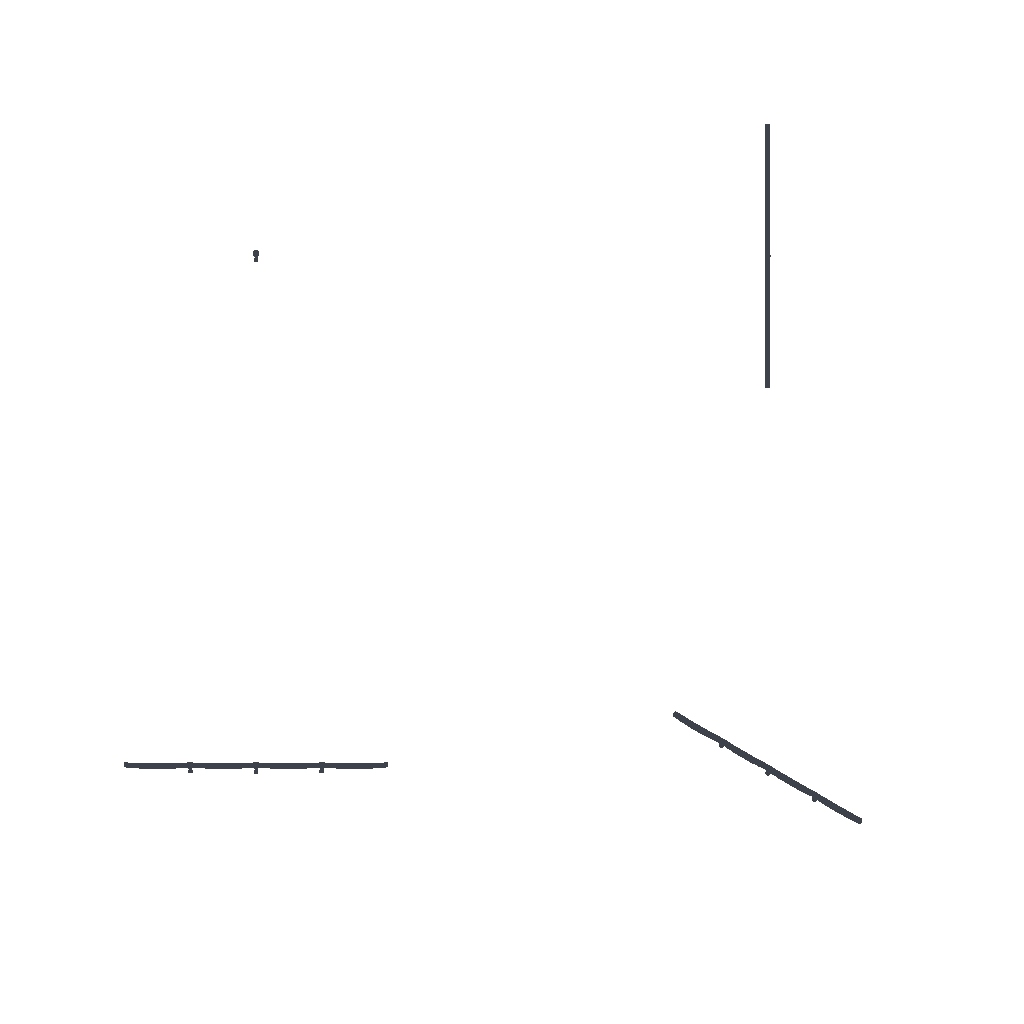Simulation study | abaqus
Set-up summary, first 274 of 540 lines:
category,name,step,type,value,unit,region
solver,abaqus,,Abaqus/CAE 2024
units,mm-N-s-tonne (MPa),,inferred,E=103600 density=6.967e-09
analysis,Step-G,,static,nlgeom=True; time_period=1
analysis,Step-F,,frequency (modal),n_modes=6
mesh,nodes,,,45210
mesh,elements,,,48438
element_type,B31,,,45138
element_type,T3D2,,,3300
material,conductor,,E,103600
material,conductor,,nu,0.3
material,conductor,,density,6.967e-09
material,ground,,E,103600
material,ground,,nu,0.3
material,ground,,density,6.967e-09
material,insulator,,E,206000
material,insulator,,nu,0.3
material,insulator,,density,1.9108e-09
material,insulator,,yield,2548
material,insulator,,cte,1.55e+07
material,insulator,,behaviors,plastic; expansion
material,steel-235,,E,206000
material,steel-235,,nu,0.3
material,steel-235,,density,7.85e-09
material,steel-235,,yield,235
material,steel-235,,behaviors,plastic
material,steel-355,,E,206000
material,steel-355,,nu,0.3
material,steel-355,,density,7.85e-09
material,steel-355,,yield,355
material,steel-355,,behaviors,plastic
material,steel-420,,E,206000
material,steel-420,,nu,0.3
material,steel-420,,density,7.85e-09
material,steel-420,,yield,420
material,steel-420,,behaviors,plastic
section,conductor,,solid section,,,_PickedSet2
section,conductor,,solid section,,,_PickedSet2
section,conductor,,solid section,,,_PickedSet2
section,ground,,solid section,,,_PickedSet2
section,steel-235,,beam section,,,_I1
section,steel-235,,beam section,,,_I2
section,steel-355,,beam section,,,_I3
section,steel-355,,beam section,,,_I4
section,steel-355,,beam section,,,_I5
section,steel-355,,beam section,,,_I6
section,steel-355,,beam section,,,_I7
section,steel-355,,beam section,,,_I8
section,steel-235,,beam section,,,_I9
section,steel-235,,beam section,,,_I10
section,steel-235,,beam section,,,_I11
section,steel-355,,beam section,,,_I12
section,steel-355,,beam section,,,_I13
section,steel-355,,beam section,,,_I14
section,steel-355,,beam section,,,_PickedSet581
section,steel-235,,beam section,,,_I16
section,steel-355,,beam section,,,_PickedSet580
section,steel-235,,beam section,,,_I18
section,steel-355,,beam section,,,_I19
section,steel-355,,beam section,,,_I20
section,steel-355,,beam section,,,_I21
section,steel-355,,beam section,,,_I22
section,steel-355,,beam section,,,_I23
section,steel-355,,beam section,,,_I24
section,steel-355,,beam section,,,_I25
section,steel-355,,beam section,,,_I26
section,steel-235,,beam section,,,_I27
section,steel-235,,beam section,,,_I28
section,steel-235,,beam section,,,_I29
section,steel-235,,beam section,,,_I30
section,steel-235,,beam section,,,_I31
section,steel-355,,beam section,,,_I32
section,steel-355,,beam section,,,_I33
section,steel-355,,beam section,,,_I34
section,steel-355,,beam section,,,_I35
section,steel-355,,beam section,,,_I36
section,steel-355,,beam section,,,_I37
section,steel-355,,beam section,,,_I38
section,steel-355,,beam section,,,_I39
section,steel-355,,beam section,,,_I40
section,steel-355,,beam section,,,_I41
section,steel-235,,beam section,,,_I42
section,steel-235,,beam section,,,_PickedSet576
section,steel-235,,beam section,,,_PickedSet577
section,steel-355,,beam section,,,_I45
section,steel-355,,beam section,,,_I46
section,steel-235,,beam section,,,_I47
section,steel-235,,beam section,,,_PickedSet579
section,steel-355,,beam section,,,_I49
section,steel-355,,beam section,,,_I50
section,steel-235,,beam section,,,_PickedSet603
section,steel-235,,beam section,,,_PickedSet604
section,steel-235,,beam section,,,_I53
section,steel-235,,beam section,,,_I54
section,steel-355,,beam section,,,_I55
section,steel-235,,beam section,,,_I56
section,steel-235,,beam section,,,_I57
section,steel-355,,beam section,,,_I58
section,steel-355,,beam section,,,_I59
section,steel-235,,beam section,,,_I60
section,steel-235,,beam section,,,_I61
section,steel-355,,beam section,,,_I62
section,steel-355,,beam section,,,_I63
section,steel-235,,beam section,,,_I64
section,steel-355,,beam section,,,_I65
section,steel-355,,beam section,,,_I66
section,steel-355,,beam section,,,_I67
section,steel-235,,beam section,,,_I68
section,steel-355,,beam section,,,_I69
section,steel-235,,beam section,,,_I70
section,steel-235,,beam section,,,_I71
section,steel-355,,beam section,,,_I72
section,steel-235,,beam section,,,_PickedSet563
section,steel-355,,beam section,,,_I74
section,steel-235,,beam section,,,_I75
section,steel-235,,beam section,,,_I76
section,steel-235,,beam section,,,_I77
section,steel-355,,beam section,,,_I78
section,steel-355,,beam section,,,_PickedSet557
section,steel-355,,beam section,,,_PickedSet558
section,steel-235,,beam section,,,_I81
section,steel-355,,beam section,,,_I82
section,steel-355,,beam section,,,_I83
section,steel-235,,beam section,,,_I84
section,steel-355,,beam section,,,_I85
section,steel-355,,beam section,,,_I86
section,steel-355,,beam section,,,_I87
section,steel-235,,beam section,,,_I88
section,steel-235,,beam section,,,_I89
section,steel-235,,beam section,,,_I90
section,steel-355,,beam section,,,_I91
section,steel-235,,beam section,,,_I92
section,steel-235,,beam section,,,_I93
section,steel-235,,beam section,,,_I94
section,steel-235,,beam section,,,_I95
section,steel-235,,beam section,,,_I96
section,steel-235,,beam section,,,_I97
section,steel-355,,beam section,,,_I98
section,steel-355,,beam section,,,_I99
section,steel-355,,beam section,,,_I100
section,steel-355,,beam section,,,_I101
section,steel-355,,beam section,,,_I102
section,steel-355,,beam section,,,_I103
section,steel-235,,beam section,,,_I104
section,steel-235,,beam section,,,_I105
section,steel-355,,beam section,,,_I106
section,steel-235,,beam section,,,_I107
section,steel-355,,beam section,,,_I108
section,steel-235,,beam section,,,_I109
section,steel-235,,beam section,,,_I110
section,steel-355,,beam section,,,_I111
section,steel-235,,beam section,,,_I112
section,steel-235,,beam section,,,_I113
section,steel-355,,beam section,,,_I114
section,steel-355,,beam section,,,_I115
section,steel-235,,beam section,,,_I116
section,steel-235,,beam section,,,_I117
section,steel-235,,beam section,,,_I118
section,steel-235,,beam section,,,_I119
section,steel-235,,beam section,,,_I120
section,steel-235,,beam section,,,_I121
section,steel-235,,beam section,,,_I122
section,steel-235,,beam section,,,_I123
section,steel-355,,beam section,,,_I124
section,steel-420,,beam section,,,_I125
section,steel-355,,beam section,,,_I126
section,steel-355,,beam section,,,_I127
section,steel-355,,beam section,,,_I128
section,steel-420,,beam section,,,_I129
section,steel-355,,beam section,,,_I130
section,steel-235,,beam section,,,_I131
section,steel-235,,beam section,,,_I132
section,steel-355,,beam section,,,_I133
section,steel-355,,beam section,,,_I134
section,steel-235,,beam section,,,_I135
section,steel-235,,beam section,,,_I136
section,steel-235,,beam section,,,_I137
section,steel-235,,beam section,,,_I138
section,steel-235,,beam section,,,_I139
section,steel-235,,beam section,,,_I140
section,steel-235,,beam section,,,_I141
section,steel-355,,beam section,,,_I142
section,steel-235,,beam section,,,_I143
section,steel-235,,beam section,,,_I144
section,steel-235,,beam section,,,_I145
section,steel-235,,beam section,,,_I146
section,steel-235,,beam section,,,_I147
section,steel-235,,beam section,,,_I148
section,steel-355,,beam section,,,_I149
section,steel-235,,beam section,,,_I150
section,steel-235,,beam section,,,_I151
section,steel-235,,beam section,,,_I152
section,steel-235,,beam section,,,_I153
section,steel-235,,beam section,,,_I154
section,steel-235,,beam section,,,_I155
section,steel-235,,beam section,,,_I156
section,steel-235,,beam section,,,_I157
section,steel-355,,beam section,,,_I158
section,steel-235,,beam section,,,_I159
section,steel-235,,beam section,,,_I160
section,steel-235,,beam section,,,_I161
section,steel-355,,beam section,,,_I162
section,steel-235,,beam section,,,_I163
section,steel-235,,beam section,,,_I164
section,steel-355,,beam section,,,_I165
section,steel-235,,beam section,,,_I166
section,steel-355,,beam section,,,_I167
section,steel-355,,beam section,,,_I168
section,steel-355,,beam section,,,_I169
section,steel-235,,beam section,,,_I170
section,steel-235,,beam section,,,_I171
section,steel-355,,beam section,,,_I172
section,steel-355,,beam section,,,_I173
section,steel-235,,beam section,,,_I174
section,steel-355,,beam section,,,_I175
section,steel-235,,beam section,,,_I176
section,steel-235,,beam section,,,_I177
section,steel-235,,beam section,,,_I178
section,steel-235,,beam section,,,_I179
section,steel-235,,beam section,,,_I180
section,steel-355,,beam section,,,_I181
section,steel-355,,beam section,,,_I182
section,steel-235,,beam section,,,_I183
section,steel-235,,beam section,,,_I184
section,steel-235,,beam section,,,_I185
section,steel-355,,beam section,,,_I186
section,steel-235,,beam section,,,_I187
section,steel-235,,beam section,,,_I188
section,steel-235,,beam section,,,_I189
section,steel-235,,beam section,,,_I190
section,steel-235,,beam section,,,_I191
section,steel-355,,beam section,,,_I192
section,steel-235,,beam section,,,_I193
section,steel-235,,beam section,,,_I194
section,steel-355,,beam section,,,_I195
section,steel-355,,beam section,,,_I196
section,steel-235,,beam section,,,_PickedSet553
section,steel-235,,beam section,,,_I198
section,steel-355,,beam section,,,_I199
section,steel-235,,beam section,,,_I200
section,steel-355,,beam section,,,_I201
section,steel-235,,beam section,,,_I202
section,steel-235,,beam section,,,_I203
section,steel-355,,beam section,,,_I204
section,steel-420,,beam section,,,_I205
section,steel-355,,beam section,,,_PickedSet542
section,steel-355,,beam section,,,_I207
section,steel-235,,beam section,,,_PickedSet535
section,steel-235,,beam section,,,_PickedSet534
section,steel-355,,beam section,,,_I210
section,steel-420,,beam section,,,_I211
section,steel-355,,beam section,,,_I212
section,steel-235,,beam section,,,_PickedSet536
section,steel-420,,beam section,,,_I214
section,steel-355,,beam section,,,_I215
section,steel-420,,beam section,,,_I216
section,steel-235,,beam section,,,_I217
section,steel-235,,beam section,,,_PickedSet514
section,steel-235,,beam section,,,_I219
section,steel-235,,beam section,,,_I220
section,steel-235,,beam section,,,_I221
section,steel-235,,beam section,,,_I222
section,steel-235,,beam section,,,_I223
section,steel-235,,beam section,,,_I224
section,steel-355,,beam section,,,_I225
section,steel-420,,beam section,,,_I226
section,steel-235,,beam section,,,_I227
section,steel-235,,beam section,,,_I228
section,steel-355,,beam section,,,_I229
section,steel-235,,beam section,,,_I230
section,steel-235,,beam section,,,_I231
section,steel-235,,beam section,,,_I232
section,steel-235,,beam section,,,_I233
section,steel-235,,beam section,,,_I234
Abaqus input file, long lists of numbers shortened, first 686 of 3467 lines:
*Heading
** Job name: deck Model name: Model-1
** Generated by: Abaqus/CAE 2024
*Preprint, echo=NO, model=NO, history=NO, contact=NO
**
** PARTS
**
*Part, name=conductor-1
*Node
      1,    -199300.5,   5545.472,           0.
      2,  -195326.375,   5107.127,           0.
** (99 more lines like these left out)
*Element, type=T3D2
  1,   1,   2
  2,   2,   3
** (98 more lines like these left out)
*Nset, nset=_PickedSet2, internal, generate
   1,  101,    1
*Elset, elset=_PickedSet2, internal, generate
   1,  100,    1
** Section: conductor
*Solid Section, elset=_PickedSet2, material=conductor
425.24,
*End Part
**
*Part, name=conductor-2
*Node
      1,    -199305.5,   5545.75,           0.
      2,  -195331.281,   5107.384,           0.
** (99 more lines like these left out)
*Element, type=T3D2
  1,   1,   2
  2,   2,   3
** (98 more lines like these left out)
*Nset, nset=_PickedSet2, internal, generate
   1,  101,    1
*Elset, elset=_PickedSet2, internal, generate
   1,  100,    1
** Section: conductor
*Solid Section, elset=_PickedSet2, material=conductor
425.24,
*End Part
**
*Part, name=conductor-3
*Node
      1,  -199120.688,   5535.459,           0.
      2,  -195150.125,   5097.904,           0.
** (99 more lines like these left out)
*Element, type=T3D2
  1,   1,   2
  2,   2,   3
** (98 more lines like these left out)
*Nset, nset=_PickedSet2, internal, generate
   1,  101,    1
*Elset, elset=_PickedSet2, internal, generate
   1,  100,    1
** Section: conductor
*Solid Section, elset=_PickedSet2, material=conductor
425.24,
*End Part
**
*Part, name=ground
*Node
      1,  -199400.406,    2214.142,           0.
      2,  -195410.953,   2038.688,           0.
** (99 more lines like these left out)
*Element, type=T3D2
  1,   1,   2
  2,   2,   3
** (98 more lines like these left out)
*Nset, nset=_PickedSet2, internal, generate
   1,  101,    1
*Elset, elset=_PickedSet2, internal, generate
   1,  100,    1
** Section: ground
*Solid Section, elset=_PickedSet2, material=ground
148.07,
*End Part
**
*Part, name=shudianta
*Node
      1,  -2504.131,   915.163,       45600.
      2,       -3822.,   683.185,   46098.164
** (13957 more lines like these left out)
*Element, type=B31
1,   1, 715
2, 715, 716
** (15044 more lines like these left out)
*Nset, nset=Wire-2-Set-1
   506,   511,   515,   517,   550,   552,   556,   557,   570,   573,   575,   576,   584,   586,   587,   589
   593,   594,   596,   600,   607,   619,   620,   622,   627,   628,   641,   644,   646,   648,   653,   655
** (33 more lines like these left out)
*Elset, elset=Wire-2-Set-1
  8915,  8916,  8917,  8918,  8919,  8920,  8921,  8922,  8923,  8924, 10205, 10206, 10207, 10208, 10209, 10210
 10211, 10212, 10213, 10214, 10215, 10216, 10217, 10218, 10219, 10220, 10221, 10222, 10223, 10224, 10478, 10479
** (33 more lines like these left out)
*Nset, nset=Wire-3-Set-1
   503,   516,   517,   558,   559,   560,   561,   563,   570,   571,   573,   575,   580,   581,   582,   583
   584,   586,   587,   589,   590,   591,   593,   594,   596,   600,   601,   619,   620,   622,   623,   624
** (37 more lines like these left out)
*Elset, elset=Wire-3-Set-1
  8939,  8940,  8941,  8942,  8943,  8944,  8945,  8946,  8947,  8948,  8949,  8950, 10239, 10240, 10241, 10242
 10243, 10244, 10245, 10246, 10247, 10248, 10249, 10250, 10251, 10252, 10253, 10254, 10255, 10256, 10257, 10258
** (35 more lines like these left out)
*Nset, nset=Wire-4-Set-1
   516,   558,   559,   560,   561,   562,   563,   571,   581,   582,   583,   591,   592,   601,   602,   623
   624,   626,   638,   643,   649,   650,   651,   652,   668,   669,   670,   683,   684,   690,   698,   705
** (13 more lines like these left out)
*Elset, elset=Wire-4-Set-1
 10263, 10264, 10265, 10266, 10267, 10268, 10269, 10270, 10271, 10272, 10273, 10274, 10275, 10276, 10285, 10286
 10287, 10288, 10297, 10298, 10299, 10300, 10301, 10302, 10303, 10304, 10305, 10306, 10698, 10699, 10700, 10701
** (12 more lines like these left out)
*Nset, nset=Wire-5-Set-1
   506,   507,   508,   509,   510,   511,   573,   574,   575,   641,   642,   644,   646,   688,   689,   691
   692,   693,   694,   697,   707,  8321,  8322,  8323,  8324,  8325,  8326,  8327,  8328,  8329,  8330,  8340
** (13 more lines like these left out)
*Elset, elset=Wire-5-Set-1
  8826,  8827,  8828,  8829,  8830,  8831,  8832,  8833,  8834,  8835,  8836,  8847,  8848,  8849,  8850,  8851
  8852,  8853,  8854,  8855,  8856,  8857,  8858,  8859,  8860,  8861,  8862,  8863,  8864,  8865,  8866,  8867
** (13 more lines like these left out)
*Nset, nset=Wire-6-Set-1
   507,   508,   510,   557,   574,   576,  8331,  8332,  8333,  8334,  8335,  8336,  8337,  8338,  8339,  9960
  9961,  9962,  9963,  9964,  9965,  9966, 11238, 11239, 11240, 11241, 11242, 11243, 11244, 11245, 11246, 11247
** (2 more lines like these left out)
*Elset, elset=Wire-6-Set-1
  8837,  8838,  8839,  8840,  8841,  8842,  8843,  8844,  8845,  8846, 10620, 10621, 10622, 10623, 10624, 10625
 10626, 10627, 12024, 12025, 12026, 12027, 12028, 12029, 12030, 12031, 12032, 12033, 12034, 12168, 12169, 12170
** (2 more lines like these left out)
*Nset, nset=Wire-7-Set-1
   511,   517,   518,   577,   584,   585,   586,   587,   588,   589,   593,   594,   595,   596,   597,   600
   607,   659,   661,   702,   703,  8434,  8435,  8436,  8437,  8438,  8439,  8440,  9976,  9977,  9978,  9979
** (13 more lines like these left out)
*Elset, elset=Wire-7-Set-1
  8951,  8952,  8953,  8954,  8955,  8956,  8957,  8958, 10638, 10639, 10640, 10641, 10642, 10643, 10644, 10645
 10646, 10647, 10648, 10735, 10736, 10737, 10738, 10739, 10740, 10741, 10742, 10743, 10744, 10745, 10746, 10747
** (13 more lines like these left out)
*Nset, nset=Wire-8-Set-1
   515,   518,   577,   660,   702,   703,  8441,  8442,  8443,  8444,  8445,  8446,  8447,  8448,  8449,  8450
  9986,  9987,  9988,  9989,  9990,  9991,  9992, 10330, 10331, 10332, 10333, 10334, 10335, 10336, 10337, 10338
** (2 more lines like these left out)
*Elset, elset=Wire-8-Set-1
  8959,  8960,  8961,  8962,  8963,  8964,  8965,  8966,  8967,  8968,  8969, 10649, 10650, 10651, 10652, 10653
 10654, 10655, 10656, 11031, 11032, 11033, 11034, 11035, 11036, 11037, 11038, 11039, 11040, 14288, 14289, 14290
** (2 more lines like these left out)
*Nset, nset=Wire-9-Set-1
   550,   607,   615,   616,   617,   618,   619,   620,   621,   622,   627,   666,   671,   672,   677,   678
   679,   680,   681,   682,   706, 10610, 10611, 10612, 10613, 10614, 10615, 10616, 10617, 10618, 10619, 10629
** (13 more lines like these left out)
*Elset, elset=Wire-9-Set-1
 11338, 11339, 11340, 11341, 11342, 11343, 11344, 11345, 11346, 11347, 11348, 11359, 11360, 11361, 11362, 11363
 11364, 11365, 11366, 11367, 11368, 11369, 11370, 11371, 11372, 11373, 11374, 11375, 11376, 11377, 11378, 11379
** (13 more lines like these left out)
*Nset, nset=Wire-10-Set-1
   615,   616,   618,   628,   665,   666, 10620, 10621, 10622, 10623, 10624, 10625, 10626, 10627, 10628, 10768
 10769, 10770, 10771, 10772, 10773, 10774, 12204, 12205, 12206, 12207, 12208, 12209, 12210, 12287, 12288, 12289
** (2 more lines like these left out)
*Elset, elset=Wire-10-Set-1
 11349, 11350, 11351, 11352, 11353, 11354, 11355, 11356, 11357, 11358, 11512, 11513, 11514, 11515, 11516, 11517
 11518, 11519, 13088, 13089, 13090, 13091, 13092, 13093, 13094, 13095, 13179, 13180, 13181, 13182, 13183, 13184
** (2 more lines like these left out)
*Nset, nset=Wire-11-Set-1
   506,   550,   551,   553,   554,   555,   569,   570,   648,   653,   655,   656,   685,   686,   687,   699
   700,   701,   709,   711,   713,  9531,  9532,  9533,  9534,  9535,  9536,  9537,  9538,  9539,  9540,  9558
** (13 more lines like these left out)
*Elset, elset=Wire-11-Set-1
 10148, 10149, 10150, 10151, 10152, 10153, 10154, 10155, 10156, 10157, 10158, 10178, 10179, 10180, 10181, 10182
 10183, 10184, 10185, 10186, 10187, 10188, 10189, 10190, 10191, 10192, 10193, 10459, 10460, 10461, 10462, 10463
** (13 more lines like these left out)
*Nset, nset=Wire-12-Set-1
   551,   552,   553,   555,   556,   569,  9541,  9542,  9543,  9544,  9545,  9546,  9547,  9548,  9549,  9550
  9551,  9552,  9553,  9554,  9555,  9556,  9557,  9572,  9573,  9574,  9575,  9576,  9577,  9578,  9579,  9580
** (2 more lines like these left out)
*Elset, elset=Wire-12-Set-1
 10159, 10160, 10161, 10162, 10163, 10164, 10165, 10166, 10167, 10168, 10169, 10170, 10171, 10172, 10173, 10174
 10175, 10176, 10177, 10194, 10195, 10196, 10197, 10198, 10199, 10200, 10201, 10202, 10203, 10204, 10470, 10471
** (2 more lines like these left out)
*Nset, nset=Wire-13-Set-1
   504,   505,   506,   511,   512,   514,   550,   566,   568,   578,   579,   598,   607,   608,   609,   611
   612,   613,   614,   634,   635,   636,   639,   647,  8312,  8313,  8314,  8315,  8316,  8317,  8318,  8319
** (13 more lines like these left out)
*Elset, elset=Wire-13-Set-1
  8816,  8817,  8818,  8819,  8820,  8821,  8822,  8823,  8824,  8825,  8877,  8878,  8879,  8880,  8881,  8882
  8883,  8884,  8885,  8886,  8905,  8906,  8907,  8908,  8909,  8910,  8911,  8912,  8913,  8914, 10449, 10450
** (13 more lines like these left out)
*Nset, nset=Wire-14-Set-1
   503,   504,   505,   512,   513,   514,   566,   567,   568,   578,   579,   580,   598,   608,   609,   610
   611,   612,   613,   614,   630,   632,   634,   635,   636,   637,   639,   647,  8307,  8308,  8309,  8310
** (10 more lines like these left out)
*Elset, elset=Wire-14-Set-1
  8810,  8811,  8812,  8813,  8814,  8815,  8887,  8888,  8889,  8890,  8891,  8892,  8893,  8894,  8895,  8896
  8897,  8898,  8899,  8900,  8901,  8902,  8903,  8904, 10415, 10416, 10417, 10418, 10419, 10420, 10440, 10441
** (9 more lines like these left out)
*Nset, nset=Wire-15-Set-1
   506,   511,   513,   550,   567,   607,   610,   637,  9792,  9793,  9794,  9795, 10207, 10208, 10209, 10210
 12249, 12250, 12251, 12252, 12735, 12736, 12737, 12738
*Elset, elset=Wire-15-Set-1
 10435, 10436, 10437, 10438, 10439, 10895, 10896, 10897, 10898, 10899, 13137, 13138, 13139, 13140, 13141, 13675
 13676, 13677, 13678, 13679
*Nset, nset=Wire-18-Set-1
   436,   451,   452,   469,   470,   471,   473,   477,   483,   484,   487,   488,   489,   490,   492,   494
   495,   496,   498,   499,   524,   525,   529,   535,  7425,  7426,  7427,  7428,  7429,  7430,  7431,  7432
** (8 more lines like these left out)
*Elset, elset=Wire-18-Set-1
  7823,  7824,  7825,  7826,  7827,  7828,  7829,  7830,  7831,  8365,  8366,  8367,  8368,  8369,  8370,  8371
  8372,  8373,  8374,  8375,  8376,  8377,  8378,  8379,  8380,  8381,  8382,  8383,  8384,  8587,  8588,  8589
** (8 more lines like these left out)
*Nset, nset=Wire-19-Set-1
   456,   502,   506,   511,   538,   548,   549,   550,   565,   572,   605,   606,   607,   629,   631,   667
  8264,  8265,  8266,  8267,  8268,  8269,  8270,  8271,  8272,  8273,  8274,  8275,  8276,  8277,  9503,  9504
** (13 more lines like these left out)
*Elset, elset=Wire-19-Set-1
  8764,  8765,  8766,  8767,  8768,  8769,  8770,  8771,  8772,  8773,  8774,  8775,  8776,  8777,  8778, 10118
 10119, 10120, 10121, 10122, 10123, 10124, 10125, 10126, 10127, 10128, 10129, 10130, 10131, 10132, 10133, 10134
** (13 more lines like these left out)
*Nset, nset=Wire-20-Set-1
   502,   503,   549,   564,   565,   572,   580,   606,   629,   630,   631,   632,   633,   658,   664,   667
  8278,  8279,  8280,  8281,  8282,  8283,  8284,  8285,  8286,  8287,  8288,  8289,  8290,  8291,  8292,  8293
** (14 more lines like these left out)
*Elset, elset=Wire-20-Set-1
  8779,  8780,  8781,  8782,  8783,  8784,  8785,  8786,  8787,  8788,  8789,  8790,  8791,  8792,  8793,  8794
  8795, 10325, 10326, 10327, 10328, 10329, 10330, 10331, 10332, 10333, 10334, 10335, 10336, 10337, 10338, 10339
** (14 more lines like these left out)
*Nset, nset=Wire-21-Set-1
   453,   454,   455,   456,   460,   478,   479,   481,   497,   501,   519,   520,   521,   522,   527,   531
   532,   534,   536,   538,   539,   541,   543,   544,   547,   548,   603,   605,  7187,  7188,  7189,  7190
** (27 more lines like these left out)
*Elset, elset=Wire-21-Set-1
  7560,  7561,  7562,  7563,  7564,  7565,  7566,  7567,  7568,  7569,  7570,  7571,  7572,  7590,  7591,  7592
  7593,  7594,  7595,  7596,  7597,  7598,  7599,  7600,  7601,  7602,  7603,  7604,  7605,  7691,  7692,  7693
** (27 more lines like these left out)
*Nset, nset=Wire-22-Set-1
   454,   455,   458,   460,   479,   481,   482,   519,   521,   522,   531,   534,   536,   537,   539,   543
   544,   546,   547,   603,  7199,  7200,  7201,  7202,  7203,  7204,  7205,  7206,  7207,  7208,  7209,  7210
** (21 more lines like these left out)
*Elset, elset=Wire-22-Set-1
  7573,  7574,  7575,  7576,  7577,  7578,  7579,  7580,  7581,  7582,  7583,  7584,  7585,  7586,  7587,  7588
  7589,  7626,  7627,  7628,  7629,  7630,  7631,  7632,  7633,  7634,  7635,  7636,  7637,  7638,  7659,  7660
** (21 more lines like these left out)
*Nset, nset=Wire-23-Set-1
   454,   455,   457,   459,   460,   479,   480,   481,   519,   521,   522,   531,   533,   534,   536,   539
   540,   542,   543,   544,   545,   547,   603,   604,  7238,  7239,  7240,  7241,  7242,  7243,  7244,  7245
** (10 more lines like these left out)
*Elset, elset=Wire-23-Set-1
  7615,  7616,  7617,  7618,  7619,  7620,  7621,  7622,  7623,  7624,  7625,  7648,  7649,  7650,  7651,  7652
  7653,  7654,  7655,  7656,  7657,  7658,  8301,  8302,  8303,  8304,  8305,  8306,  8307,  8308,  8309,  8310
** (9 more lines like these left out)
*Nset, nset=Wire-26-Set-1
   372,   373,   374,   376,   377,   400,   401,   403,   404,   406,   434,   461,   462,   464,   465,   466
   467,   474,   475,   485,   486,   500,   523,   528,  5247,  5248,  5249,  5250,  5251,  5252,  5253,  5283
** (6 more lines like these left out)
*Elset, elset=Wire-26-Set-1
  5307,  5308,  5309,  5310,  5311,  5312,  5313,  5314,  5347,  5348,  5349,  5350,  5351,  5352,  5353,  5354
  5355,  5356,  5357,  5358,  5359,  5360,  7108,  7109,  7110,  7111,  7112,  7113,  7114,  7115,  7500,  7501
** (6 more lines like these left out)
*Nset, nset=Wire-27-Set-1
  222,  224,  260,  261,  262,  349,  351,  368,  371,  378,  379,  399,  408,  410,  427,  463
 3742, 3743, 3744, 3745, 3746, 3747, 3748, 3749, 3750, 3751, 3752, 3753, 3754, 3755, 3756, 3757
** (7 more lines like these left out)
*Elset, elset=Wire-27-Set-1
 3545, 3546, 3547, 3548, 3549, 3550, 3551, 3552, 3553, 3554, 3555, 3556, 3557, 3558, 3559, 3560
 3561, 3562, 5290, 5291, 5292, 5293, 5294, 5295, 5296, 5297, 5298, 5373, 5374, 5375, 5376, 5377
** (7 more lines like these left out)
*Nset, nset=Wire-28-Set-1
  203,  215,  221,  222,  223,  224,  259,  261,  263,  349,  350,  351,  368,  408,  409,  410
 3030, 3031, 3032, 3033, 3034, 3035, 3036, 3037, 3038, 3039, 3040, 3041, 3042, 3043, 3044, 3045
** (5 more lines like these left out)
*Elset, elset=Wire-28-Set-1
 2709, 2710, 2711, 2712, 2713, 2714, 2715, 2716, 2717, 2718, 2719, 2720, 2721, 2722, 2723, 2724
 2725, 2726, 2727, 2728, 2729, 2730, 2731, 2732, 2733, 2734, 2735, 2736, 4921, 4922, 4923, 4924
** (5 more lines like these left out)
*Nset, nset=Wire-29-Set-1
  262,  370,  378,  379,  399,  407,  426,  433, 5817, 5818, 5819, 5820, 5821, 5822, 5823, 6745
 6746, 6747, 6748, 6749, 6750, 6751, 6752, 6753, 6754, 6755, 6756, 6757, 6758, 6769, 6770, 6771
** (2 more lines like these left out)
*Elset, elset=Wire-29-Set-1
 5970, 5971, 5972, 5973, 5974, 5975, 5976, 5977, 7049, 7050, 7051, 7052, 7053, 7054, 7055, 7056
 7057, 7058, 7059, 7060, 7061, 7062, 7063, 7064, 7076, 7077, 7078, 7079, 7080, 7081, 7082, 7083
** (2 more lines like these left out)
*Nset, nset=Wire-30-Set-1
  203,  215,  221,  263,  370,  407,  426,  433, 5225, 5226, 5227, 5228, 5229, 5230, 5231, 5824
 5825, 5826, 5827, 5828, 5829, 5830, 6485, 6486, 6487, 6488, 6489, 6490, 6491, 6492, 6493, 6494
** (2 more lines like these left out)
*Elset, elset=Wire-30-Set-1
 5282, 5283, 5284, 5285, 5286, 5287, 5288, 5289, 5978, 5979, 5980, 5981, 5982, 5983, 5984, 5985
 6755, 6756, 6757, 6758, 6759, 6760, 6761, 6762, 6763, 6764, 6765, 6766, 6767, 6768, 6769, 6770
** (2 more lines like these left out)
*Nset, nset=Wire-31-Set-1
  197,  200,  201,  202,  203,  204,  205,  206,  207,  211,  212,  213,  214,  215,  216,  217
  218,  219,  220,  221,  263,  265,  266,  267,  335,  346,  347,  352, 2890, 2891, 2892, 2893
** (12 more lines like these left out)
*Elset, elset=Wire-31-Set-1
 2545, 2546, 2547, 2548, 2549, 2550, 2551, 2552, 2553, 2554, 2555, 2556, 2557, 2558, 2559, 2560
 2561, 2562, 2563, 2564, 2565, 2566, 2567, 2568, 2569, 2570, 2571, 2572, 2573, 2574, 2575, 2576
** (12 more lines like these left out)
*Nset, nset=Wire-32-Set-1
  200,  202,  204,  212,  214,  217,  219,  220,  225,  258,  264,  265,  266,  335,  346,  347
  348,  352, 3061, 3062, 3063, 3064, 3065, 3066, 3775, 3776, 3777, 3778, 3779, 3780, 3781, 3782
** (8 more lines like these left out)
*Elset, elset=Wire-32-Set-1
 2745, 2746, 2747, 2748, 2749, 2750, 2751, 3582, 3583, 3584, 3585, 3586, 3587, 3588, 3589, 3590
 3591, 3592, 3593, 3594, 3595, 3596, 4702, 4703, 4704, 4705, 4706, 4707, 4708, 4709, 4710, 4711
** (8 more lines like these left out)
*Nset, nset=Wire-33-Set-1
  192,  193,  194,  195,  196,  197,  207,  211,  218,  273,  329,  330,  331,  336,  338,  369
  394,  424, 2849, 2850, 2851, 2852, 2853, 2854, 2855, 2856, 2857, 2858, 2859, 2860, 2861, 2862
** (5 more lines like these left out)
*Elset, elset=Wire-33-Set-1
 2497, 2498, 2499, 2500, 2501, 2502, 2503, 2504, 2505, 2506, 2507, 2508, 2509, 2510, 2511, 2512
 2513, 2514, 2515, 2516, 2517, 2518, 2519, 2520, 4639, 4640, 4641, 4642, 4643, 4644, 4645, 4646
** (4 more lines like these left out)
*Nset, nset=Wire-34-Set-1
  194,  196,  257,  329,  331,  333,  336,  337,  338,  356,  369,  424, 4705, 4706, 4707, 4708
 4709, 4756, 4757, 4758, 4759, 4760, 4761, 4762, 4763, 4764, 4765, 4766, 4767, 4768, 4769, 4770
** (3 more lines like these left out)
*Elset, elset=Wire-34-Set-1
 4677, 4678, 4679, 4680, 4681, 4682, 4737, 4738, 4739, 4740, 4741, 4742, 4743, 4744, 4745, 4746
 4747, 4748, 4749, 4750, 4751, 4752, 4753, 4754, 5257, 5258, 5259, 5260, 5261, 5262, 5263, 5264
** (3 more lines like these left out)
*Nset, nset=Wire-35-Set-1
  188,  189,  191,  192,  193,  251,  252,  253,  271,  273,  313,  324,  325,  326,  327,  390
  392,  394,  395,  396,  397,  398,  411,  412,  420,  422,  423,  449, 2802, 2803, 2804, 2805
** (9 more lines like these left out)
*Elset, elset=Wire-35-Set-1
 2443, 2444, 2445, 2446, 2447, 2460, 2461, 2462, 2463, 2464, 3470, 3471, 3472, 3473, 3474, 3481
 3482, 3483, 3484, 3485, 3486, 4560, 4561, 4562, 4563, 4564, 4565, 4566, 4567, 4568, 4569, 4570
** (9 more lines like these left out)
*Nset, nset=Wire-36-Set-1
  189,  190,  191,  252,  253,  272,  324,  327,  390,  391,  392,  395,  397,  398,  411,  412
  420,  421,  422,  423, 2806, 2807, 2808, 2809, 2810, 2811, 2812, 2813, 2814, 2815, 3683, 3684
** (7 more lines like these left out)
*Elset, elset=Wire-36-Set-1
 2448, 2449, 2450, 2451, 2452, 2453, 2454, 2455, 2456, 2457, 2458, 2459, 3475, 3476, 3477, 3478
 3479, 3480, 4554, 4555, 4556, 4557, 4558, 4559, 4571, 4572, 4573, 4574, 4575, 4581, 4582, 4583
** (7 more lines like these left out)
*Nset, nset=Wire-37-Set-1
  149,  164,  179,  180,  182,  186,  187,  188,  251,  271,  288,  289,  298,  302,  303,  304
  311,  312,  313,  314,  317,  318,  319,  320,  323,  415,  416,  418, 2736, 2737, 2738, 2739
** (9 more lines like these left out)
*Elset, elset=Wire-37-Set-1
 2365, 2366, 2367, 2368, 2369, 2382, 2383, 2384, 2385, 2386, 2426, 2427, 2428, 2429, 2430, 2437
 2438, 2439, 2440, 2441, 2442, 3948, 3949, 3950, 3951, 3952, 3965, 3966, 3967, 3968, 3969, 4234
** (9 more lines like these left out)
*Nset, nset=Wire-38-Set-1
  180,  181,  182,  186,  187,  250,  288,  289,  302,  304,  311,  312,  314,  315,  317,  320
  322,  323,  415,  418, 2740, 2741, 2742, 2743, 2744, 2745, 2746, 2747, 2748, 2749, 2792, 2793
** (7 more lines like these left out)
*Elset, elset=Wire-38-Set-1
 2370, 2371, 2372, 2373, 2374, 2375, 2376, 2377, 2378, 2379, 2380, 2381, 2431, 2432, 2433, 2434
 2435, 2436, 3953, 3954, 3955, 3956, 3957, 3958, 3959, 3960, 3961, 3962, 3963, 3964, 4360, 4361
** (7 more lines like these left out)
*Nset, nset=Wire-39-Set-1
   68,   71,   72,   74,   76,  130,  132,  146,  147,  149,  162,  163,  164,  165,  167,  169
  179,  268,  269,  270,  287,  298,  307,  308,  309,  310,  419,  476, 1347, 1348, 1349, 1350
** (8 more lines like these left out)
*Elset, elset=Wire-39-Set-1
  738,  739,  740,  741,  742,  753,  754,  755,  756,  757, 1628, 1629, 1630, 1631, 1632, 1643
 1644, 1645, 1646, 1647, 1971, 1972, 1973, 1974, 1975, 2084, 2085, 2086, 2087, 2088, 2095, 2096
** (8 more lines like these left out)
*Nset, nset=Wire-40-Set-1
   72,   73,   74,  130,  131,  132,  146,  163,  167,  168,  169,  268,  270,  287,  305,  307
  309,  310,  419,  476, 1351, 1352, 1353, 1354, 1355, 1356, 1357, 1358, 2114, 2115, 2116, 2117
** (6 more lines like these left out)
*Elset, elset=Wire-40-Set-1
  743,  744,  745,  746,  747,  748,  749,  750,  751,  752, 1633, 1634, 1635, 1636, 1637, 1638
 1639, 1640, 1641, 1642, 1965, 1966, 1967, 1968, 1969, 1970, 2079, 2080, 2081, 2082, 2083, 2089
** (6 more lines like these left out)
*Nset, nset=Wire-41-Set-1
  147,  148,  183,  269, 2406, 2407, 2408, 2409, 2410, 6147, 6148, 6149, 6150, 6151
*Elset, elset=Wire-41-Set-1
 1976, 1977, 1978, 1979, 1980, 1981, 6356, 6357, 6358, 6359, 6360, 6361
*Nset, nset=Wire-42-Set-1
   10,   33,   38,   62,   63,   64,   65,   66,   67,   68,   71,   76,   77,   79,   80,   82
   83,   84,   85,   86,   87,   88,  109,  110,  111,  112,  113,  114,  119,  123,  124,  125
** (18 more lines like these left out)
*Elset, elset=Wire-42-Set-1
  676,  677,  678,  679,  680,  688,  689,  690,  691,  692,  693,  694,  695,  696,  697,  698
  699,  700,  701,  702,  703,  704,  705,  706,  707,  708,  709,  710,  711,  712,  780,  781
** (18 more lines like these left out)
*Nset, nset=Wire-43-Set-1
   12,   14,   17,   20,   22,   24,   26,   28,   40,   41,   42,   43,   44,   45,   46,   61
  101,  105,  106,  172,  176,  232,  233, 1087, 1088, 1089, 1090, 1101, 1102, 1103, 1104, 1105
** (7 more lines like these left out)
*Elset, elset=Wire-43-Set-1
  433,  434,  435,  436,  437,  450,  451,  452,  453,  454,  455,  456,  457,  458,  459,  499
  500,  501,  502,  503,  504,  505,  506,  507, 1114, 1115, 1116, 1117, 1118, 1203, 1204, 1205
** (7 more lines like these left out)
*Nset, nset=Wire-44-Set-1
   10,   33,   38,   41,   43,   82,  101,  172, 1091, 1092, 1093, 1094, 1668, 1669, 1670, 1671
 1854, 1855, 1856, 1857, 3498, 3499, 3500, 3501
*Elset, elset=Wire-44-Set-1
  438,  439,  440,  441,  442, 1109, 1110, 1111, 1112, 1113, 1324, 1325, 1326, 1327, 1328, 3253
 3254, 3255, 3256, 3257
*Nset, nset=Wire-45-Set-1
   68,   71,   75,   76,  148,  165,  183,  184,  185,  290,  291,  321,  417, 1363, 1364, 1365
 1366, 1367, 1368, 1369, 1370, 1371, 1372, 1373, 1374, 1375, 1376, 1377, 1378, 1379, 1380, 1381
** (4 more lines like these left out)
*Elset, elset=Wire-45-Set-1
  758,  759,  760,  761,  762,  763,  764,  765,  766,  767,  768,  769,  770,  771,  772,  773
  774,  775,  776,  777,  778,  779, 1954, 1955, 1956, 1957, 1958, 1959, 1960, 1961, 1962, 1963
** (4 more lines like these left out)
*Nset, nset=Wire-46-Set-1
  149,  164,  179,  184,  185,  290,  298,  417, 4106, 4107, 4108, 4109, 4110, 4326, 4327, 4328
 4329, 4330, 4556, 4557, 4558, 4559, 4560, 6137, 6138, 6139, 6140, 6141
*Elset, elset=Wire-46-Set-1
 3970, 3971, 3972, 3973, 3974, 3975, 4228, 4229, 4230, 4231, 4232, 4233, 4502, 4503, 4504, 4505
 4506, 4507, 6344, 6345, 6346, 6347, 6348, 6349
*Nset, nset=Wire-47-Set-1
  192,  193,  198,  199,  208,  210,  273,  332,  339,  341,  353,  354,  394, 2875, 2876, 2877
 2878, 2879, 2880, 4692, 4693, 4694, 4695, 4696, 4697, 4698, 4699, 4700, 4701, 4702, 4703, 4704
** (6 more lines like these left out)
*Elset, elset=Wire-47-Set-1
 2528, 2529, 2530, 2531, 2532, 2533, 2534, 4663, 4664, 4665, 4666, 4667, 4668, 4669, 4670, 4671
 4672, 4673, 4674, 4675, 4676, 4761, 4762, 4763, 4764, 4765, 4766, 4767, 4778, 4779, 4780, 4781
** (5 more lines like these left out)
*Nset, nset=Wire-48-Set-1
  197,  198,  207,  208,  209,  210,  211,  218,  340,  341, 2869, 2870, 2871, 2872, 2873, 2874
 2938, 2939, 2940, 2941, 2942, 2943, 2944, 2945, 2946, 2947, 2948, 2949, 2950, 2951, 2952, 2953
** (2 more lines like these left out)
*Elset, elset=Wire-48-Set-1
 2521, 2522, 2523, 2524, 2525, 2526, 2527, 2601, 2602, 2603, 2604, 2605, 2606, 2607, 2608, 2609
 2610, 2611, 2612, 2613, 2614, 2615, 2616, 2617, 2618, 2619, 2620, 2621, 2622, 2623, 2624, 4768
** (1 more lines like these left out)
*Nset, nset=Wire-49-Set-1
   65,   67,   77,   78,   79,   80,   87,   88,  129,  144,  145,  170,  177,  178,  226,  241
  247,  248,  249,  306, 1387, 1388, 1389, 1390, 1391, 1392, 1393, 1394, 1395, 1396, 1397, 1398
** (7 more lines like these left out)
*Elset, elset=Wire-49-Set-1
  785,  786,  787,  788,  789,  790,  791,  792,  793,  794,  795,  796,  797,  798,  799,  800
  801, 1916, 1917, 1918, 1919, 1920, 1921, 1922, 1923, 1924, 1925, 1926, 1927, 1928, 1929, 1930
** (7 more lines like these left out)
*Nset, nset=Wire-50-Set-1
   62,   63,   83,   85,  109,  110,  112,  114,  119,  120,  122,  123,  125,  127,  128,  141
  142,  239,  240,  245, 1299, 1300, 1301, 1302, 1303, 1304, 1968, 1969, 1970, 1971, 1972, 1973
** (7 more lines like these left out)
*Elset, elset=Wire-50-Set-1
  681,  682,  683,  684,  685,  686,  687, 1460, 1461, 1462, 1463, 1464, 1465, 1466, 1467, 1468
 1469, 1879, 1880, 1881, 1882, 1883, 1884, 1885, 1886, 1887, 1888, 1889, 1890, 1891, 1892, 1893
** (7 more lines like these left out)
*Nset, nset=Wire-51-Set-1
   22,   23,   24,   25,   26,   27,   28,   46,   61,  103,  105,  233,  871,  872,  873,  874
  875,  876,  877,  878,  879,  880,  881,  882,  883,  884,  885,  886,  887,  888,  889,  890
** (6 more lines like these left out)
*Elset, elset=Wire-51-Set-1
  182,  183,  184,  185,  186,  187,  188,  189,  190,  191,  192,  193,  194,  195,  196,  197
  198,  199,  200,  201,  202,  203,  204,  205,  206,  207,  208,  209,  210,  211,  212,  213
** (6 more lines like these left out)
*Nset, nset=Wire-52-Set-1
   12,   14,   17,   20,   21,   22,   28,   35,   36,   46,   61,  102,  859,  860,  861,  862
  863,  864,  865,  866,  867,  868,  869,  870, 1023, 1024, 1025, 1026, 1027, 1028, 1029, 1030
** (5 more lines like these left out)
*Elset, elset=Wire-52-Set-1
  168,  169,  170,  171,  172,  173,  174,  175,  176,  177,  178,  179,  180,  181,  359,  360
  361,  362,  363,  364,  365,  366,  367,  368,  369,  370,  371,  372,  373,  374,  375,  376
** (5 more lines like these left out)
*Nset, nset=Wire-53-Set-1
   10,   12,   14,   17,   20,   33,   34,   38,   39,   82, 1009, 1010, 1011, 1012, 1013, 1014
 1015, 1016, 1017, 1018, 1019, 1020, 1021, 1022, 1076, 1077, 1078, 1079, 1080, 1081, 1082, 1151
** (3 more lines like these left out)
*Elset, elset=Wire-53-Set-1
  343,  344,  345,  346,  347,  348,  349,  350,  351,  352,  353,  354,  355,  356,  357,  358
  420,  421,  422,  423,  424,  425,  426,  427,  508,  509,  510,  511,  512,  513,  514,  515
** (2 more lines like these left out)
*Nset, nset=Wire-54-Set-1
   34,   39,   40,   44, 1083, 1084, 1085, 1086, 3232, 3233, 3234, 3235
*Elset, elset=Wire-54-Set-1
  428,  429,  430,  431,  432, 2947, 2948, 2949, 2950, 2951
*Nset, nset=Wire-58-Set-1
   22,   28,  107,  235,  385,  386,  443,  444,  446,  448, 1776, 1777, 1778, 1779, 1780, 1781
 1782, 1783, 3346, 3347, 3348, 3349, 3350, 3351, 3352, 3353, 5503, 5504, 5505, 5506, 5507, 5508
** (3 more lines like these left out)
*Elset, elset=Wire-58-Set-1
 1234, 1235, 1236, 1237, 1238, 1239, 1240, 1241, 1242, 3076, 3077, 3078, 3079, 3080, 3081, 3082
 3083, 3084, 5601, 5602, 5603, 5604, 5605, 5606, 5607, 5608, 5609, 5618, 5619, 5620, 5621, 5622
** (3 more lines like these left out)
*Nset, nset=Wire-59-Set-1
   46,   48,   50,   52,   54,   56,   61,  133,  134,  135, 1246, 1247, 1248, 1249, 1250, 1251
 1252, 1253, 1267, 1268, 1269, 1270, 1271, 1272, 1273, 1274, 2201, 2202, 2203, 2204, 2205, 2206
** (3 more lines like these left out)
*Elset, elset=Wire-59-Set-1
  620,  621,  622,  623,  624,  625,  626,  627,  628,  644,  645,  646,  647,  648,  649,  650
  651,  652, 1735, 1736, 1737, 1738, 1739, 1740, 1741, 1742, 1743, 1759, 1760, 1761, 1762, 1763
** (3 more lines like these left out)
*Nset, nset=Wire-60-Set-1
   24,   26,   54,   55,   56,   57,   58,   59,   60,  105,  136,  137,  138,  139,  140,  233
  236,  237,  383,  384,  438,  439,  440,  441,  442,  446,  447,  448, 1214, 1215, 1216, 1217
** (10 more lines like these left out)
*Elset, elset=Wire-60-Set-1
  582,  583,  584,  585,  586,  587,  588,  589,  590,  591,  601,  602,  603,  604,  605,  606
  607,  608,  609,  610, 1788, 1789, 1790, 1791, 1792, 1793, 1794, 1795, 1796, 1797, 1798, 1799
** (10 more lines like these left out)
*Nset, nset=Wire-62-Set-1
   24,   26,  107,  235,  236,  384,  385,  386,  438,  439,  441,  442,  443,  444, 1764, 1765
 1766, 1767, 1768, 1769, 1770, 1771, 1772, 1773, 1774, 1775, 3334, 3335, 3336, 3337, 3338, 3339
** (5 more lines like these left out)
*Elset, elset=Wire-62-Set-1
 1221, 1222, 1223, 1224, 1225, 1226, 1227, 1228, 1229, 1230, 1231, 1232, 1233, 3063, 3064, 3065
 3066, 3067, 3068, 3069, 3070, 3071, 3072, 3073, 3074, 3075, 5593, 5594, 5595, 5596, 5597, 5598
** (5 more lines like these left out)
*Nset, nset=Wire-64-Set-1
   48,   50,   52,   57,   59,   60,  105,  133,  134,  135,  136,  137,  138,  233, 1254, 1255
 1256, 1257, 1258, 1259, 1260, 1261, 1262, 1263, 1264, 1265, 1266, 2209, 2210, 2211, 2212, 2213
** (5 more lines like these left out)
*Elset, elset=Wire-64-Set-1
  629,  630,  631,  632,  633,  634,  635,  636,  637,  638,  639,  640,  641,  642,  643, 1744
 1745, 1746, 1747, 1748, 1749, 1750, 1751, 1752, 1753, 1754, 1755, 1756, 1757, 1758, 1768, 1769
** (5 more lines like these left out)
*Nset, nset=Wire-65-Set-1
   22,   28,   46,   47,   48,   49,   50,   51,   52,   53,   54,   56,   61,  107,  133,  134
  135,  234,  235,  238,  385,  386,  387,  443,  444,  445,  446,  448, 1171, 1172, 1173, 1174
** (11 more lines like these left out)
*Elset, elset=Wire-65-Set-1
  531,  532,  533,  534,  535,  536,  537,  538,  539,  540,  541,  542,  543,  544,  545,  546
  547,  548,  549,  550,  551,  552,  553,  554,  555,  556,  557,  558,  559,  560,  561,  562
** (11 more lines like these left out)
*Nset, nset=Wire-88-Set-1
   68,   69,   71,   76,   89,   91,   98,   99,  152,  153,  155,  160,  165,  227,  230,  294
  295,  297,  301,  380, 1325, 1326, 1327, 1328, 1329, 1330, 1331, 1529, 1530, 1531, 1532, 1533
** (7 more lines like these left out)
*Elset, elset=Wire-88-Set-1
  713,  714,  715,  716,  717,  718,  719,  720,  949,  950,  951,  952,  953,  954,  955,  956
 1029, 1030, 1031, 1032, 1033, 1034, 1035, 1036, 1054, 1055, 1056, 1057, 1058, 1059, 1060, 1061
** (6 more lines like these left out)
*Nset, nset=Wire-90-Set-1
  149,  151,  152,  153,  155,  156,  157,  159,  292,  294,  295,  296,  297,  298, 2428, 2429
 2430, 2431, 2432, 2433, 2434, 2455, 2456, 2457, 2458, 2459, 2460, 2461, 4123, 4124, 4125, 4126
** (4 more lines like these left out)
*Elset, elset=Wire-90-Set-1
 2002, 2003, 2004, 2005, 2006, 2007, 2008, 2009, 2033, 2034, 2035, 2036, 2037, 2038, 2039, 2040
 3990, 3991, 3992, 3993, 3994, 3995, 3996, 3997, 3998, 3999, 4000, 4022, 4023, 4024, 4025, 4026
** (4 more lines like these left out)
*Nset, nset=Wire-91-Set-1
  150,  151,  156,  291,  300, 2424, 2425, 2426, 2427, 4140, 4141, 4142, 4143, 4260, 4261, 4262
 4263, 6159, 6160, 6161, 6162
*Elset, elset=Wire-91-Set-1
 1997, 1998, 1999, 2000, 2001, 4009, 4010, 4011, 4012, 4013, 4148, 4149, 4150, 4151, 4152, 6370
 6371, 6372, 6373, 6374
*Nset, nset=Wire-92-Set-1
  149,  150,  151,  156,  157,  158,  159,  160,  161,  292,  296,  298,  299,  300,  301, 2419
 2420, 2421, 2422, 2423, 2469, 2470, 2471, 2472, 2473, 2474, 2475, 2476, 2477, 2478, 2486, 2487
** (4 more lines like these left out)
*Elset, elset=Wire-92-Set-1
 1991, 1992, 1993, 1994, 1995, 1996, 2049, 2050, 2051, 2052, 2053, 2054, 2055, 2056, 2057, 2058
 2059, 2060, 2069, 2070, 2071, 2072, 2073, 2074, 2075, 2076, 2077, 2078, 4133, 4134, 4135, 4136
** (4 more lines like these left out)
*Nset, nset=Wire-93-Set-1
   76,  152,  153,  154,  155,  165,  166,  293,  294,  295,  297, 2442, 2443, 2444, 2445, 2446
 2447, 2448, 2449, 2450, 2451, 2452, 2453, 2454, 2547, 2548, 2549, 2550, 2551, 2552, 2553, 2554
** (4 more lines like these left out)
*Elset, elset=Wire-93-Set-1
 2018, 2019, 2020, 2021, 2022, 2023, 2024, 2025, 2026, 2027, 2028, 2029, 2030, 2031, 2032, 2140
 2141, 2142, 2143, 2144, 2145, 2146, 2147, 2148, 2149, 2150, 2151, 2152, 2153, 2154, 2155, 2156
** (5 more lines like these left out)
*Nset, nset=Wire-95-Set-1
   92,   93,   94,   95,   96,   97,  100,  229,  230,  231,  321,  380,  381,  382, 1554, 1555
 1556, 1557, 1558, 1559, 1560, 1561, 1562, 1563, 1571, 1572, 1573, 1574, 1575, 1576, 1577, 1578
** (4 more lines like these left out)
*Elset, elset=Wire-95-Set-1
  978,  979,  980,  981,  982,  983,  984,  985,  986,  987,  988,  989,  998,  999, 1000, 1001
 1002, 1003, 1004, 1005, 1006, 1007, 1008, 1009, 1010, 1011, 1012, 1085, 1086, 1087, 1088, 1089
** (4 more lines like these left out)
*Nset, nset=Wire-96-Set-1
   69,   89,   91,   92,   94,   95,   97,   98,   99,  100,  164,  179,  227,  229,  231,  382
 1549, 1550, 1551, 1552, 1553, 1591, 1592, 1593, 1594, 1595, 1596, 1597, 1605, 1606, 1607, 1608
** (5 more lines like these left out)
*Elset, elset=Wire-96-Set-1
  972,  973,  974,  975,  976,  977, 1021, 1022, 1023, 1024, 1025, 1026, 1027, 1028, 1037, 1038
 1039, 1040, 1041, 1042, 1043, 1044, 1045, 1046, 1047, 1048, 1049, 1050, 1051, 1052, 1053, 1077
** (5 more lines like these left out)
*Nset, nset=Wire-97-Set-1
   68,   69,   70,   71,   89,   90,   91,   98,   99,  227,  228, 1332, 1333, 1334, 1335, 1336
 1337, 1338, 1339, 1340, 1341, 1342, 1343, 1344, 1345, 1346, 1536, 1537, 1538, 1539, 1540, 1541
** (4 more lines like these left out)
*Elset, elset=Wire-97-Set-1
  721,  722,  723,  724,  725,  726,  727,  728,  729,  730,  731,  732,  733,  734,  735,  736
  737,  957,  958,  959,  960,  961,  962,  963,  964,  965,  966,  967,  968,  969,  970,  971
** (5 more lines like these left out)
*Nset, nset=Wire-104-Set-1
  207,  211,  357,  358,  359,  361,  365,  428,  431,  432, 5040, 5041, 5042, 5043, 5044, 5045
 5046, 5047, 5048, 5049, 5058, 5059, 5060, 5061, 5062, 5063, 5064, 5065, 6556, 6557, 6558, 6559
** (3 more lines like these left out)
*Elset, elset=Wire-104-Set-1
 5068, 5069, 5070, 5071, 5072, 5073, 5074, 5075, 5076, 5077, 5078, 5088, 5089, 5090, 5091, 5092
 5093, 5094, 5095, 5096, 6835, 6836, 6837, 6838, 6839, 6840, 6841, 6842, 6843, 6844, 6845, 6923
** (2 more lines like these left out)
*Nset, nset=Wire-105-Set-1
  353,  359,  360,  361,  362,  363,  364,  365,  366,  367,  432, 5066, 5067, 5068, 5069, 5070
 5071, 5072, 5073, 5074, 5075, 5076, 5077, 5078, 5079, 5080, 5081, 5082, 5083, 5084, 5085, 5086
** (4 more lines like these left out)
*Elset, elset=Wire-105-Set-1
 5097, 5098, 5099, 5100, 5101, 5102, 5103, 5104, 5105, 5106, 5107, 5108, 5109, 5110, 5111, 5112
 5113, 5114, 5115, 5116, 5117, 5118, 5119, 5120, 5121, 5122, 5123, 5124, 5125, 5165, 5166, 5167
** (4 more lines like these left out)
*Nset, nset=Wire-106-Set-1
  207,  211,  366,  367, 5119, 5120, 5121, 5122, 5123, 5124, 6584, 6585, 6586, 6587, 6588, 6589
*Elset, elset=Wire-106-Set-1
 5158, 5159, 5160, 5161, 5162, 5163, 5164, 6866, 6867, 6868, 6869, 6870, 6871, 6872
*Nset, nset=Wire-107-Set-1
  193,  357,  358,  394,  428,  429,  430,  431, 6601, 6602, 6603, 6604, 6605, 6606, 6607, 6608
 6609, 6610, 6611, 6612, 6613, 6614, 6615, 6616, 6617, 6618, 6619, 6620, 6621, 6622, 6623, 6624
** (4 more lines like these left out)
*Elset, elset=Wire-107-Set-1
 6886, 6887, 6888, 6889, 6890, 6891, 6892, 6893, 6894, 6895, 6896, 6897, 6898, 6899, 6900, 6901
 6902, 6903, 6904, 6905, 6906, 6907, 6908, 6909, 6910, 6911, 6912, 6913, 6914, 6915, 6916, 6917
** (4 more lines like these left out)
*Nset, nset=Wire-108-Set-1
  197,  218,  275,  277,  278,  279,  283,  285,  328,  413, 3903, 3904, 3905, 3945, 3946, 3947
 3948, 3949, 3950, 3951, 5953, 5954, 5955, 6022, 6023, 6024, 6025, 6026, 6027, 6028, 6042, 6043
** (3 more lines like these left out)
*Elset, elset=Wire-108-Set-1
 3732, 3733, 3734, 3735, 3781, 3782, 3783, 3784, 3785, 3786, 3787, 3788, 6129, 6130, 6131, 6132
 6209, 6210, 6211, 6212, 6213, 6214, 6215, 6216, 6232, 6233, 6234, 6235, 6236, 6237, 6238, 6239
** (2 more lines like these left out)
*Nset, nset=Wire-109-Set-1
  279,  280,  281,  282,  283,  284,  285,  339,  342,  413,  414, 3920, 3921, 3922, 3923, 3924
 3925, 3926, 3927, 3928, 3929, 3930, 3931, 3932, 3933, 3934, 3935, 3936, 3937, 3938, 3939, 3940
** (4 more lines like these left out)
*Elset, elset=Wire-109-Set-1
 3752, 3753, 3754, 3755, 3756, 3757, 3758, 3759, 3760, 3761, 3762, 3763, 3764, 3765, 3766, 3767
 3768, 3769, 3770, 3771, 3772, 3773, 3774, 3775, 3776, 3777, 3778, 3779, 3780, 4802, 4803, 4804
** (4 more lines like these left out)
*Nset, nset=Wire-110-Set-1
  197,  218,  342,  414, 4805, 4806, 4807, 4808, 4809, 4810, 5986, 5987, 5988, 5989, 5990, 5991
*Elset, elset=Wire-110-Set-1
 4795, 4796, 4797, 4798, 4799, 4800, 4801, 6167, 6168, 6169, 6170, 6171, 6172, 6173
*Nset, nset=Wire-111-Set-1
  192,  273,  274,  275,  276,  277,  278,  328, 3860, 3861, 3862, 3863, 3864, 3865, 3866, 3867
 3868, 3869, 3870, 3871, 3872, 3873, 3874, 3875, 3876, 3877, 3878, 3879, 3880, 3881, 3882, 3883
** (4 more lines like these left out)
*Elset, elset=Wire-111-Set-1
 3684, 3685, 3686, 3687, 3688, 3689, 3690, 3691, 3692, 3693, 3694, 3695, 3696, 3697, 3698, 3699
 3700, 3701, 3702, 3703, 3704, 3705, 3706, 3707, 3708, 3709, 3710, 3711, 3712, 3713, 3714, 3715
** (4 more lines like these left out)
*Nset, nset=_PickedSet437, internal
   203,   215,   221,   223,   259,   260,   263,   350,   371,   372,   375,   377,   400,   409,   427,   450
   463,   464,   466,   467,   468,   486,   493,   500,  3732,  3733,  3734,  3735,  3736,  3737,  3738,  3739
** (8 more lines like these left out)
*Elset, elset=_PickedSet437, internal
  3533,  3534,  3535,  3536,  3537,  3538,  3539,  3540,  3541,  3542,  3543,  3544,  5299,  5300,  5301,  5302
  5303,  5304,  5305,  5306,  5361,  5362,  5363,  5364,  5365,  5366,  5367,  5368,  5369,  5370,  5371,  5372
** (7 more lines like these left out)
*Nset, nset=_PickedSet439, internal
   64,   68,   71,   73,   76,   78,   86,  111,  126,  129,  131,  145,  149,  164,  165,  168
  179,  181,  188,  241,  250,  251,  271,  298,  305,  313,  315,  322, 2030, 2031, 2032, 2033
** (8 more lines like these left out)
*Elset, elset=_PickedSet439, internal
 1532, 1533, 1534, 1535, 1536, 1537, 1538, 1539, 1540, 1541, 1542, 1543, 1544, 1545, 1614, 1615
 1616, 1617, 1618, 1619, 1620, 1621, 1622, 1623, 1624, 1625, 1626, 1627, 2353, 2354, 2355, 2356
** (8 more lines like these left out)
*Nset, nset=_PickedSet440, internal
   10,   12,   14,   17,   20,   22,   24,   26,   28,   33,   38,   46,   61,   64,   82,   86
  105,  111,  120,  122,  126,  141,  233,  239, 1061, 1062, 1063, 1064, 1065, 1066, 1067, 1068
** (9 more lines like these left out)
*Elset, elset=_PickedSet440, internal
  403,  404,  405,  406,  407,  408,  409,  410,  411,  525,  526,  527,  528,  529,  530,  661
  662,  663,  664,  665,  666,  667,  668,  669,  670,  671,  672,  673,  674,  675,  874,  875
** (8 more lines like these left out)
*Nset, nset=_PickedSet442, internal
  188,  190,  192,  193,  197,  203,  207,  211,  215,  218,  221,  225,  251,  257,  258,  263
  264,  271,  272,  273,  313,  333,  337,  348,  356,  391,  394,  421, 2820, 2821, 2822, 2823
** (9 more lines like these left out)
*Elset, elset=_PickedSet442, internal
 2465, 2466, 2467, 2468, 2469, 2470, 2471, 2472, 2473, 2474, 2475, 2476, 2737, 2738, 2739, 2740
 2741, 2742, 2743, 2744, 3511, 3512, 3513, 3514, 3515, 3516, 3517, 3518, 3519, 3520, 3521, 3522
** (8 more lines like these left out)
*Nset, nset=Set-118
   14,   33,   46,   68,   86,  120,  129,  131,  179,  181,  203,  218,  233,  271,  272,  273
  348,  350,  356,  427,  466,  467,  468, 1166, 1167, 1168, 1169, 1170, 2086, 2087, 2088, 2089
** (8 more lines like these left out)
*Elset, elset=Set-118
  525,  526,  527,  528,  529,  530, 1600, 1601, 1602, 1603, 1604, 1605, 1606, 1607, 1608, 1609
 1610, 1611, 1612, 1613, 1614, 1615, 1616, 1617, 1618, 1619, 1620, 1621, 1622, 1623, 1624, 1625
** (8 more lines like these left out)
*Nset, nset=_PickedSet451, internal
   506,   511,   515,   517,   550,   552,   556,   557,   570,   573,   575,   576,   584,   586,   587,   589
   593,   594,   596,   600,   607,   619,   620,   622,   627,   628,   641,   644,   646,   648,   653,   655
** (33 more lines like these left out)
*Elset, elset=_PickedSet451, internal
  8915,  8916,  8917,  8918,  8919,  8920,  8921,  8922,  8923,  8924, 10205, 10206, 10207, 10208, 10209, 10210
 10211, 10212, 10213, 10214, 10215, 10216, 10217, 10218, 10219, 10220, 10221, 10222, 10223, 10224, 10478, 10479
** (33 more lines like these left out)
*Nset, nset=_PickedSet452, internal
   584,   586,   587,   589,   590,   594,   644,   645,   646,   653,   654,   655,   661,   663,   672,   673
   674,   675,   677,   679,   680,   681,   691,   692,   694,   695,   696,   700,   701,   704,   706,   707
** (20 more lines like these left out)
*Elset, elset=_PickedSet452, internal
 10785, 10786, 10787, 10788, 10789, 10790, 10791, 10792, 10793, 10794, 10795, 10796, 12217, 12218, 12219, 12220
Results summary:
result,odb.job_status,,,JOB_STATUS_COMPLETED_SUCCESSFULLY,"consistent, unstated (Abaqus has no unit system)"
result,steps[0].procedure,Step-G,,*STATIC,"consistent, unstated (Abaqus has no unit system)"
result,steps[0].time_period,Step-G,,1,"consistent, unstated (Abaqus has no unit system)"
result,steps[0].n_frames,Step-G,,22,"consistent, unstated (Abaqus has no unit system)"
result,steps[0].last_frame.id,Step-G,,21,"consistent, unstated (Abaqus has no unit system)"
result,steps[0].last_frame.value,Step-G,,1,"consistent, unstated (Abaqus has no unit system)"
result,steps[0].last_frame.description,Step-G,,Increment     21: Step Time =    1.000,"consistent, unstated (Abaqus has no unit system)"
result,steps[0].completed,Step-G,,True,"consistent, unstated (Abaqus has no unit system)"
result,steps[0].max_U_magnitude,Step-G,,5722.09,"consistent, unstated (Abaqus has no unit system)"
result,steps[0].max_S_mises,Step-G,,140.292,"consistent, unstated (Abaqus has no unit system)"
result,steps[0].RF_sum[1],Step-G,,-0.1868,"consistent, unstated (Abaqus has no unit system)"
result,steps[0].RF_sum[2],Step-G,,4.754,"consistent, unstated (Abaqus has no unit system)"
result,steps[0].RF_sum[3],Step-G,,991769,"consistent, unstated (Abaqus has no unit system)"
result,steps[1].procedure,Step-F,,*FREQUENCY,"consistent, unstated (Abaqus has no unit system)"
result,steps[1].time_period,Step-F,,0,"consistent, unstated (Abaqus has no unit system)"
result,steps[1].n_frames,Step-F,,7,"consistent, unstated (Abaqus has no unit system)"
result,steps[1].last_frame.id,Step-F,,1,"consistent, unstated (Abaqus has no unit system)"
result,steps[1].last_frame.value,Step-F,,6,"consistent, unstated (Abaqus has no unit system)"
result,steps[1].last_frame.description,Step-F,,Mode         6: Value =  0.8959     Freq =  0.1506     (cycles/time),"consistent, unstated (Abaqus has no unit system)"
result,steps[1].max_U_magnitude,Step-F,,1.279,"consistent, unstated (Abaqus has no unit system)"
result,steps[1].eigenfrequencies_hz[1],Step-F,,0.1501,"consistent, unstated (Abaqus has no unit system)"
result,steps[1].eigenfrequencies_hz[2],Step-F,,0.1503,"consistent, unstated (Abaqus has no unit system)"
result,steps[1].eigenfrequencies_hz[3],Step-F,,0.1505,"consistent, unstated (Abaqus has no unit system)"
result,steps[1].eigenfrequencies_hz[4],Step-F,,0.1506,"consistent, unstated (Abaqus has no unit system)"
result,steps[1].eigenfrequencies_hz[5],Step-F,,0.1506,"consistent, unstated (Abaqus has no unit system)"
result,steps[1].eigenfrequencies_hz[6],Step-F,,0.1506,"consistent, unstated (Abaqus has no unit system)"